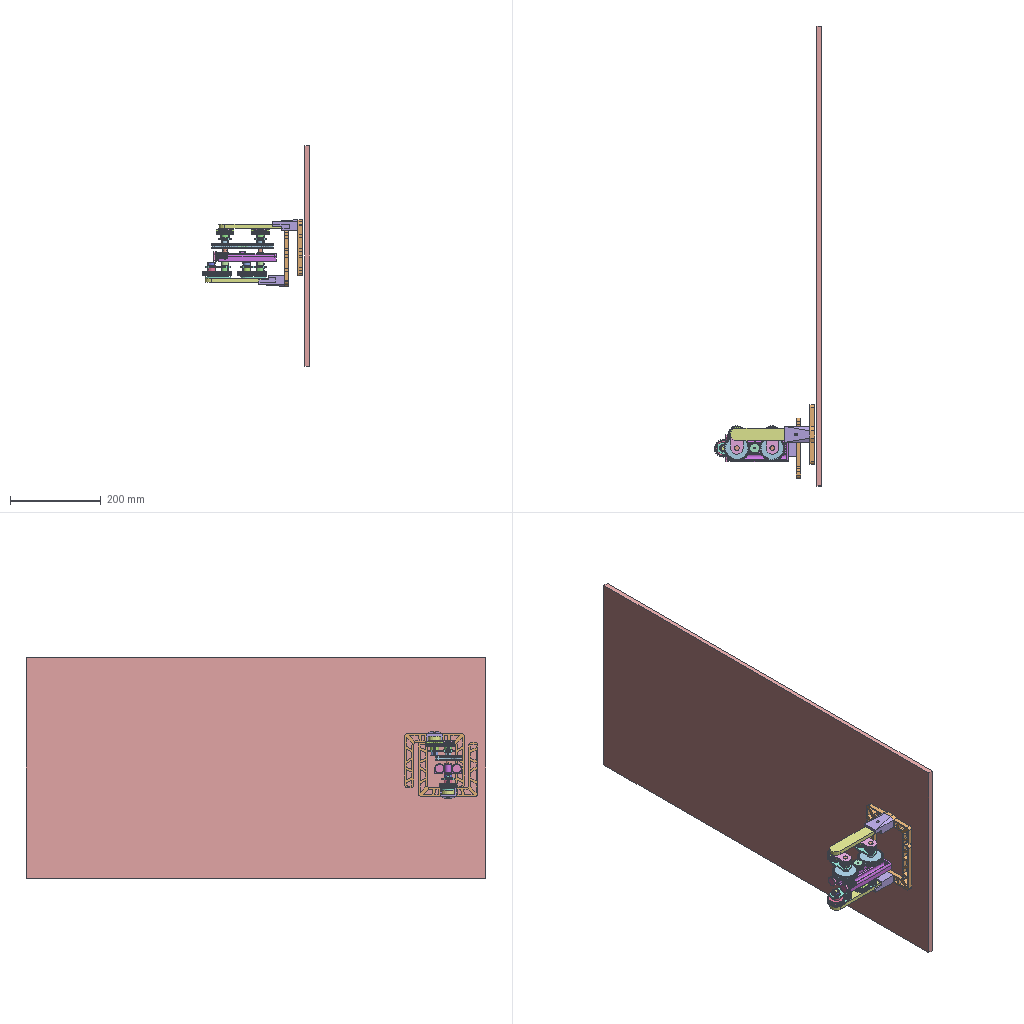Assembly | NX | 27 different items | 49 placed | box 236 x 1013 x 485 mm
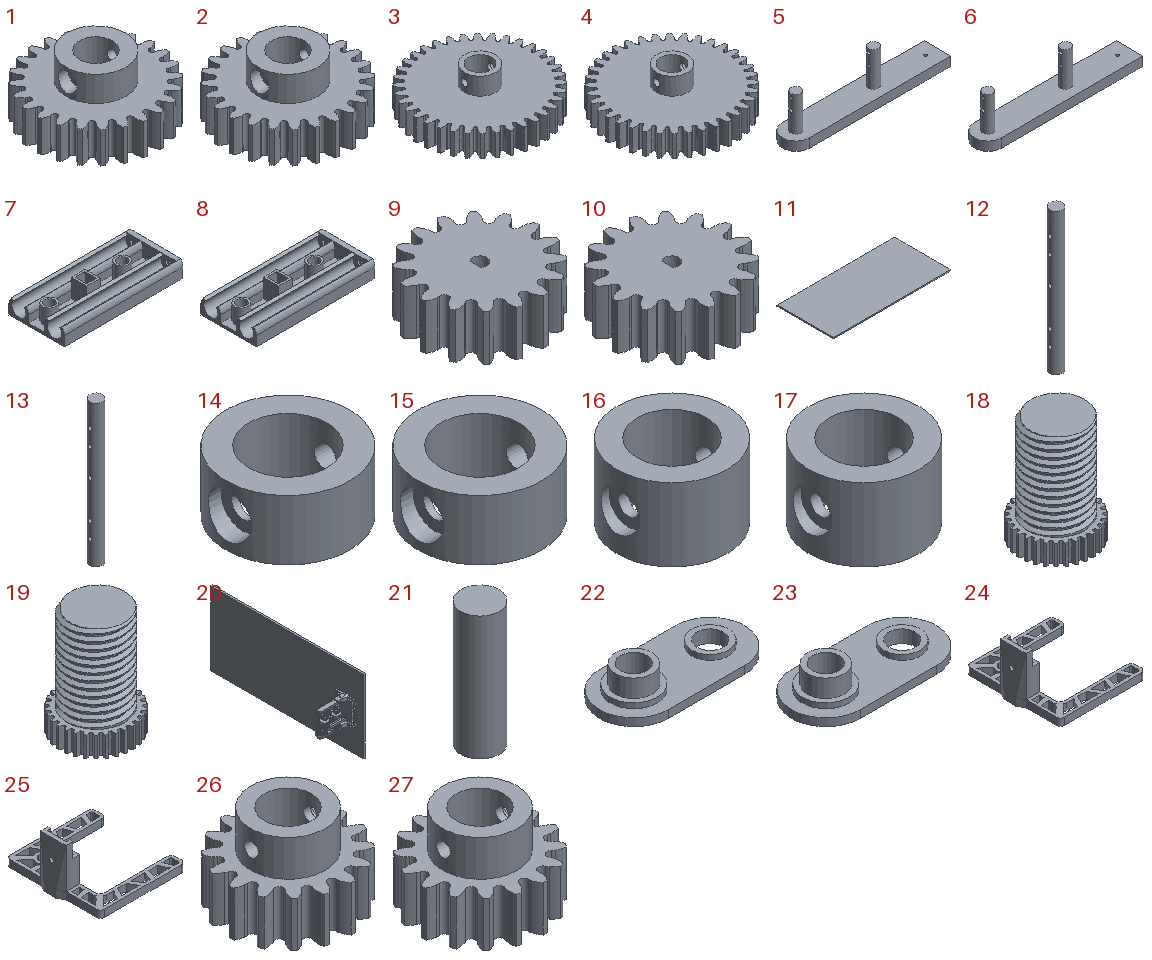Parts list (item | quantity | parent item | size | volume | features):
1 | x4 | in 20 | 38.944 x 38.944 x 18 mm | 9823 mm3 | features BREP 2, DATUM_CSYS 1, UNITE 1
2 | x1 | - | 38.944 x 38.944 x 18 mm | 9823 mm3 | features BREP 2, DATUM_CSYS 1, UNITE 1
3 | x2 | in 20 | 56.956 x 56.956 x 18 mm | 22225 mm3 | features BREP 1, DATUM_CSYS 1
4 | x1 | - | 56.956 x 56.956 x 18 mm | 22225 mm3 | features BREP 1, DATUM_CSYS 1
5 | x2 | in 20 | 155.8 x 27 x 43.5 mm | 42232 mm3 | features DATUM_CSYS 3, EXTRUDE 3, SKETCH 2, DATUM_PLANE 1
6 | x1 | - | 155.8 x 27 x 43.5 mm | 42232 mm3 | features DATUM_CSYS 3, EXTRUDE 3, SKETCH 2, DATUM_PLANE 1
7 | x1 | in 20 | 127.15 x 59.2 x 23 mm | 56788 mm3 | features EXTRUDE 5, DATUM_CSYS 4, REPLACE_FACE 4, SKETCH 3, CHAMFER 1, OFFSET 1, UNITE 1
8 | x1 | - | 127.15 x 59.2 x 23 mm | 56788 mm3 | features EXTRUDE 5, DATUM_CSYS 4, REPLACE_FACE 4, SKETCH 3, CHAMFER 1, OFFSET 1, UNITE 1
9 | x1 | in 20 | 26.979 x 26.979 x 10 mm | 4412 mm3 | features BREP 1, DATUM_CSYS 1
10 | x1 | - | 26.979 x 26.979 x 10 mm | 4412 mm3 | features BREP 1, DATUM_CSYS 1
11 | x1 | in 20 | 1013 x 485 x 10 mm | 4913050 mm3 | features DATUM_CSYS 2, EXTRUDE 1, SKETCH 1
12 | x2 | in 20 | 10 x 10 x 111.5 mm | 8408 mm3 | features DATUM_CSYS 3, EXTRUDE 2, SKETCH 2, SUBTRACT 1
13 | x1 | - | 10 x 10 x 111.5 mm | 8408 mm3 | features DATUM_CSYS 3, EXTRUDE 2, SKETCH 2, SUBTRACT 1
14 | x4 | in 20 | 16.4 x 16.4 x 8 mm | 928.38 mm3 | features BREP 1, DATUM_CSYS 1
15 | x1 | - | 16.4 x 16.4 x 8 mm | 928.38 mm3 | features BREP 1, DATUM_CSYS 1
16 | x2 | in 20 | 16.4 x 16.4 x 10.9 mm | 1304 mm3 | features BREP 1, DATUM_CSYS 1
17 | x1 | - | 16.4 x 16.4 x 10.9 mm | 1304 mm3 | features BREP 1, DATUM_CSYS 1
18 | x2 | in 20 | 21.396 x 21.396 x 31 mm | 6909 mm3 | features BREP 1, DATUM_CSYS 1, THREADS 1
19 | x1 | - | 21.396 x 21.396 x 31 mm | 6909 mm3 | features BREP 1, DATUM_CSYS 1, THREADS 1
20 | x1 | - | 235.972 x 1013 x 485 mm | 5370772 mm3 | features DATUM_CSYS 24, EXTRUDE 13, SKETCH 11, BREP 10, REPLACE_FACE 5, UNITE 3, CHAMFER 1, CYLINDER 1, DATUM_PLANE 1, OFFSET 1, SUBTRACT 1, THREADS 1
21 | x1 | - | 10.2 x 10.2 x 33 mm | 2697 mm3 | features DATUM_CSYS 2, EXTRUDE 1, SKETCH 1
22 | x8 | in 20 | 57.14 x 27.14 x 12 mm | 4732 mm3 | features DATUM_CSYS 2, EXTRUDE 2, CYLINDER 1, REPLACE_FACE 1, SKETCH 1, UNITE 1
23 | x1 | - | 57.14 x 27.14 x 12 mm | 4732 mm3 | features DATUM_CSYS 2, EXTRUDE 2, CYLINDER 1, REPLACE_FACE 1, SKETCH 1, UNITE 1
24 | x2 | in 20 | 123.846 x 131.35 x 66 mm | 70448 mm3 | features DATUM_CSYS 3, BREP 2, SKETCH 2
25 | x1 | - | 123.846 x 131.35 x 66 mm | 70448 mm3 | features DATUM_CSYS 3, BREP 2, SKETCH 2
26 | x4 | in 20 | 26.979 x 26.979 x 18 mm | 4568 mm3 | features BREP 1, DATUM_CSYS 1
27 | x1 | - | 26.979 x 26.979 x 18 mm | 4568 mm3 | features BREP 1, DATUM_CSYS 1
Mates (type | each side: item.copy, entity, surface, feature):
Touch | 24.1 face cylinder Body(2) | 5.1 face cylinder Extrude(2) | 2 times
Touch | 18.1 face cylinder Body(1) | 7.1 face cylinder Extrude(5) | 2 times
Distance | 18.1 face plane Body(1) | 7.1 face plane Extrude(5) | 2 times
Distance | 12.1 face plane Extrude(3) | 5.1 face plane Extrude(2) | 2 times
Touch | 3.1 face cylinder Body(1) | 12.1 face cylinder Extrude(4)
Touch | 3.1 face plane Body(1) | 9.1 face plane Body(1)
Touch | 9.1 face plane Body(1) | 3.1 face plane Body(1)
Touch | 26.1 face cylinder Body(1) | 12.1 face cylinder Extrude(3)
Touch | 5.1 face plane Extrude(2) | 12.1 edge
Touch | 5.1 face plane Extrude(2) | 24.1 face plane Body(2)
Touch | 24.1 face plane Body(2) | 5.1 face plane Extrude(2)
Touch | 22.1 face plane Extrude(2) | 14.1 face plane Body(1) | 2 times
Touch | 22.1 face cylinder Extrude(2) | 26.1 face cylinder Body(1)
Touch | 22.1 face plane Extrude(2) | 26.1 face plane Body(1)
Touch | 9.1 face cylinder Body(1) | 3.1 face cylinder Body(1) | 2 times